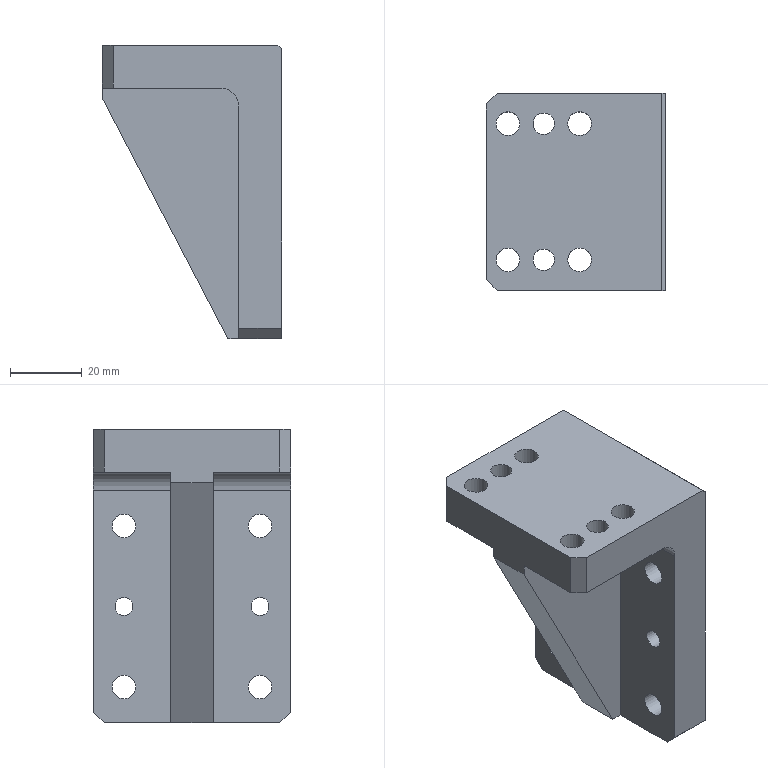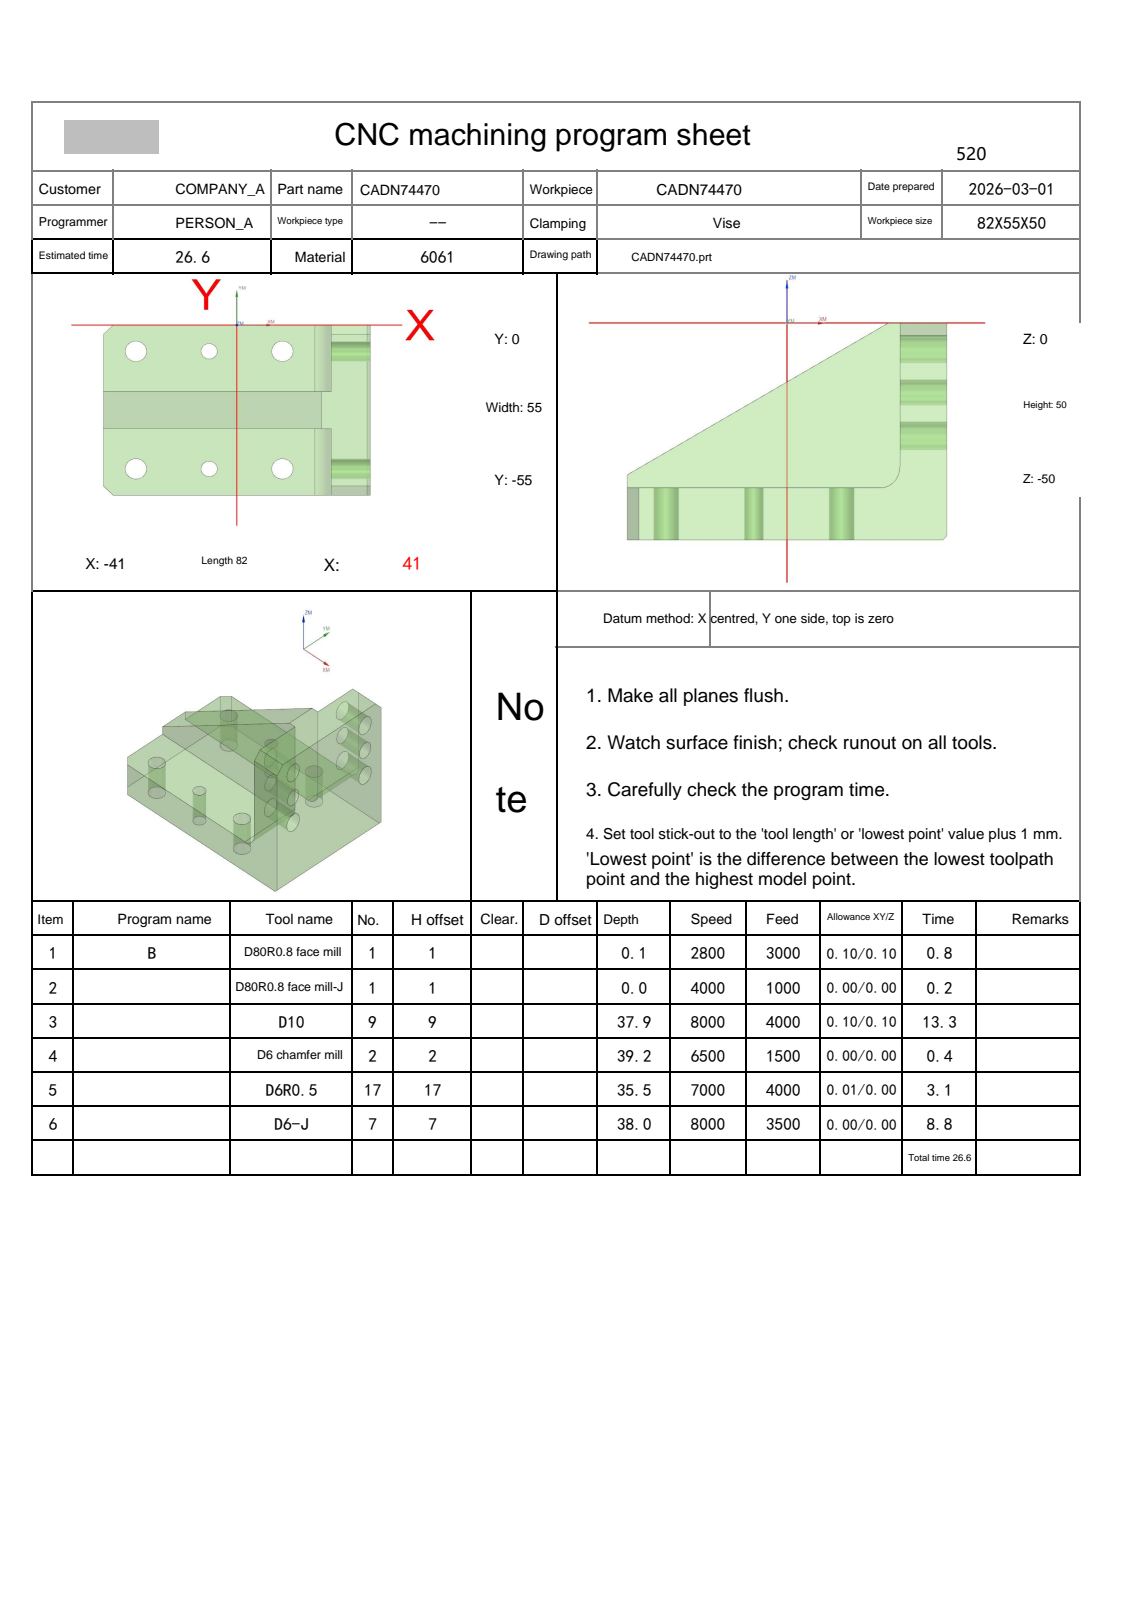NC program | NX | posted by the shop | part box 50 x 55 x 82 mm
Lines 1 to 109 of 26562:
%
O0001
(Machine time: 27.64 MIN)
(===Total Tool:5===)
(T1=D80R0.8 face mill D=80.  R=0.8  D-  H01 Z=0.    )
(T9=D10     D=10.  R=0.   D-  H09 Z=-37.9 )
(T2=D6 chamfer mill   D=6.   R=0.   D-  H02 Z=-39.2 )
(T17=D6R0.5 D=6.   R=0.5  D-  H17 Z=-35.5 )
(T7=D6-J    D=6.   R=0.   D7  H07 Z=-38.  )
G80 G90 G17 G49 G40
G91 G28 Z0
M01
N1 T01 M06
(D80R0.8 face mill  D=80. R=0.8 H=01 ce=0.10 di=0.10)
G00 G90 G54 X-93.097 Y-27.5 M03 S2800
G43 H01 Z50.
M08
Z6.011
G01 Z4.011 F3000.
X-81.097
X81.097
X93.097
Z6.011
G00 X-93.097
Z5.522
G01 Z3.522
X-81.097
X81.097
X93.097
Z5.522
G00 X-93.097
Z5.033
G01 Z3.033
X-81.097
X81.097
X93.097
Z5.033
G00 X-93.097
Z4.544
G01 Z2.544
X-81.097
X81.097
X93.097
Z4.544
G00 Z50.
X-93.097
Z4.056
G01 Z2.056
X-81.097
X81.097
X93.097
Z4.056
G00 Z50.
X-93.097
Z3.567
G01 Z1.567
X-81.097
X81.097
X93.097
Z3.567
G00 Z50.
X-93.097
Z3.078
G01 Z1.078
X-81.097
X81.097
X93.097
Z3.078
G00 Z50.
X-93.097
Z2.589
G01 Z.589
X-81.097
X81.097
X93.097
Z2.589
G00 Z50.
X-93.097
Z2.1
G01 Z.1
X-81.097
X81.097
X93.097
Z2.1
G00 Z50.
G91 G28 Z0.0
M05
M09
G91 G28 Z0.0
M01
N2 T01 M06
(D80R0.8 face mill-J  D=80. R=0.8 H=01 ce=0.00 di=0.00)
G00 G90 G54 X-92.999 Y-27.5 M03 S4000
G43 H01 Z50.
M08
Z2.
G01 Z0.0 F1000.
X-80.999
X80.999
X92.999
Z2.
G00 Z50.
G91 G28 Z0.0
M05
M09
G91 G28 Z0.0
M01